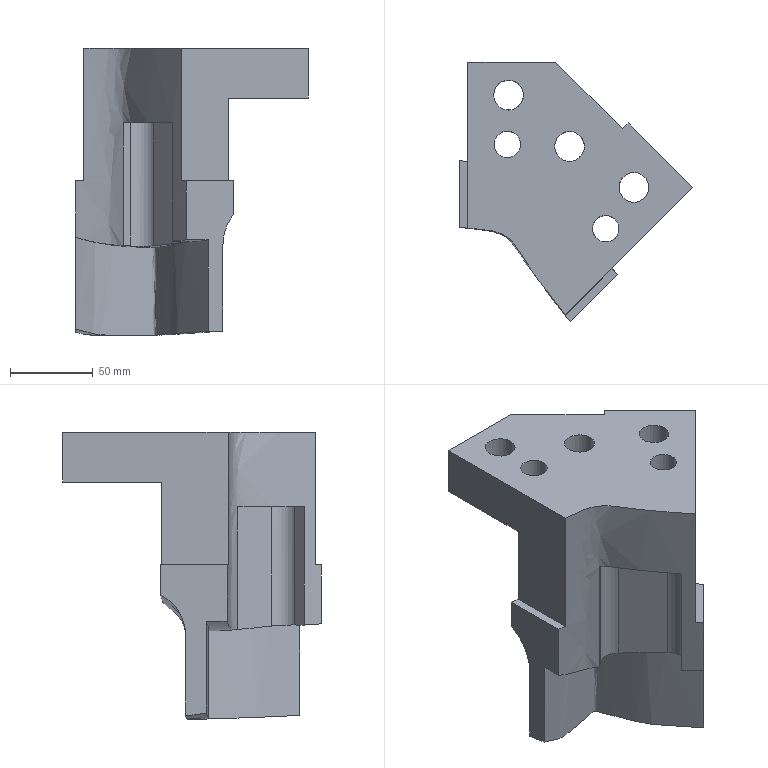Part | NX | features solid 2 | 1 solid | 38 faces | box 140.657 x 156.28 x 173.715 mm | volume 690605 mm3 | plane 19 | cylinder 10 | spline 9 | commonest cylinder face diameters 18 x3 26 x3 16 x2 20 x2